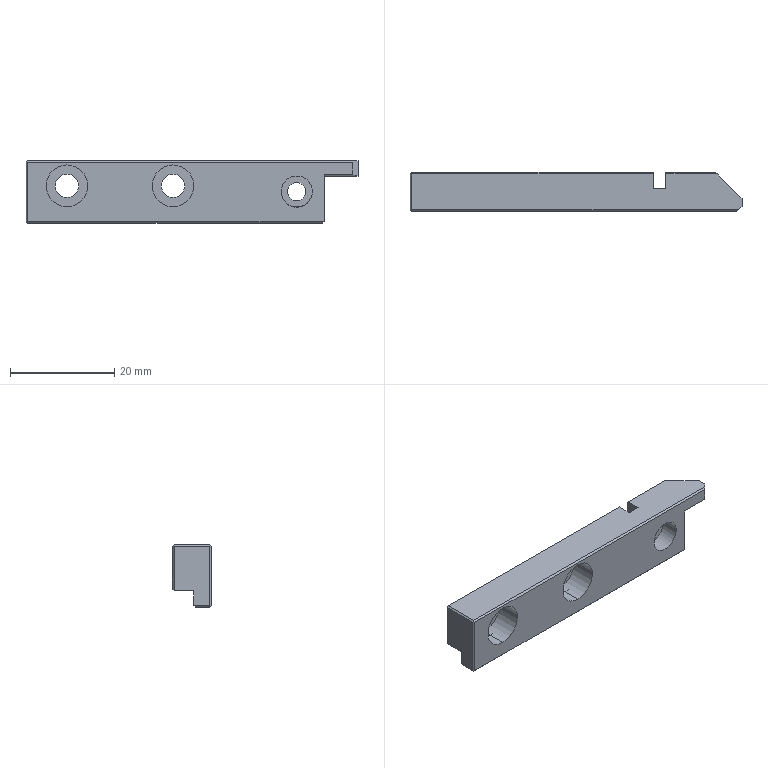Part | NX | 1 solid | 43 faces | box 63.7 x 7.5 x 11.95 mm | volume 3584 mm3 | plane 31 | cylinder 12 | commonest cylinder face diameters 4.5 x4 8 x4 3.5 x2 6 x2
STEP:
#1=CARTESIAN_POINT('',(-198.5,219.5,-37.608));
#2=VERTEX_POINT('',#1);
#3=CARTESIAN_POINT('',(-198.5,219.5,-34.742));
#4=VERTEX_POINT('',#3);
#5=CARTESIAN_POINT('',(-198.5,219.5,-36.191));
#6=DIRECTION('',(0.,0.,1.));
#7=VECTOR('',#6,1000.);
#8=LINE('',#5,#7);
#9=EDGE_CURVE('',#2,#4,#8,.T.);
#10=ORIENTED_EDGE('',*,*,#9,.T.);
#11=CARTESIAN_POINT('',(-199.2,218.8,-34.742));
#12=VERTEX_POINT('',#11);
#13=CARTESIAN_POINT('',(-196.,222.,-34.742));
#14=DIRECTION('',(0.7071,0.7071,0.));
#15=VECTOR('',#14,1000.);
#16=LINE('',#13,#15);
#17=EDGE_CURVE('',#12,#4,#16,.T.);
#18=ORIENTED_EDGE('',*,*,#17,.F.);
#19=CARTESIAN_POINT('',(-199.5,218.5,-35.042));
#20=VERTEX_POINT('',#19);
#21=CARTESIAN_POINT('',(-199.935,218.065,-35.477));
#22=DIRECTION('',(0.5774,0.5774,0.5774));
#23=VECTOR('',#22,1000.);
#24=LINE('',#21,#23);
#25=EDGE_CURVE('',#20,#12,#24,.T.);
#26=ORIENTED_EDGE('',*,*,#25,.F.);
#27=CARTESIAN_POINT('',(-199.5,218.5,-37.34));
#28=VERTEX_POINT('',#27);
#29=CARTESIAN_POINT('',(-199.5,218.5,-36.191));
#30=DIRECTION('',(0.,0.,1.));
#31=VECTOR('',#30,1000.);
#32=LINE('',#29,#31);
#33=EDGE_CURVE('',#28,#20,#32,.T.);
#34=ORIENTED_EDGE('',*,*,#33,.F.);
#35=CARTESIAN_POINT('',(-196.,222.,-38.278));
#36=DIRECTION('',(-0.6947,-0.6947,0.1862));
#37=VECTOR('',#36,1000.);
#38=LINE('',#35,#37);
#39=EDGE_CURVE('',#2,#28,#38,.T.);
#40=ORIENTED_EDGE('',*,*,#39,.F.);
#41=EDGE_LOOP('',(#10,#18,#26,#34,#40));
#42=FACE_BOUND('',#41,.T.);
#43=CARTESIAN_POINT('',(-199.,219.,-36.191));
#44=DIRECTION('',(-0.7071,0.7071,0.));
#45=DIRECTION('',(0.,0.,1.));
#46=AXIS2_PLACEMENT_3D('',#43,#44,#45);
#47=PLANE('',#46);
#48=ADVANCED_FACE('',(#42),#47,.F.);
#49=CARTESIAN_POINT('',(-262.2,218.8,-46.392));
#50=VERTEX_POINT('',#49);
#51=CARTESIAN_POINT('',(-262.2,218.8,-35.042));
#52=VERTEX_POINT('',#51);
#53=CARTESIAN_POINT('',(-262.2,218.8,-35.477));
#54=DIRECTION('',(0.,0.,1.));
#55=VECTOR('',#54,1000.);
#56=LINE('',#53,#55);
#57=EDGE_CURVE('',#50,#52,#56,.T.);
#58=ORIENTED_EDGE('',*,*,#57,.T.);
#59=CARTESIAN_POINT('',(-262.2,225.7,-35.042));
#60=VERTEX_POINT('',#59);
#61=CARTESIAN_POINT('',(-262.2,222.1,-35.042));
#62=DIRECTION('',(0.,-1.,0.));
#63=VECTOR('',#62,1000.);
#64=LINE('',#61,#63);
#65=EDGE_CURVE('',#60,#52,#64,.T.);
#66=ORIENTED_EDGE('',*,*,#65,.F.);
#67=CARTESIAN_POINT('',(-262.2,225.7,-43.542));
#68=VERTEX_POINT('',#67);
#69=CARTESIAN_POINT('',(-262.2,225.7,-39.292));
#70=DIRECTION('',(0.,0.,1.));
#71=VECTOR('',#70,1000.);
#72=LINE('',#69,#71);
#73=EDGE_CURVE('',#68,#60,#72,.T.);
#74=ORIENTED_EDGE('',*,*,#73,.F.);
#75=CARTESIAN_POINT('',(-262.2,221.9,-43.542));
#76=VERTEX_POINT('',#75);
#77=CARTESIAN_POINT('',(-262.2,222.,-43.542));
#78=DIRECTION('',(0.,1.,0.));
#79=VECTOR('',#78,1000.);
#80=LINE('',#77,#79);
#81=EDGE_CURVE('',#76,#68,#80,.T.);
#82=ORIENTED_EDGE('',*,*,#81,.F.);
#83=CARTESIAN_POINT('',(-262.2,221.9,-46.392));
#84=VERTEX_POINT('',#83);
#85=CARTESIAN_POINT('',(-262.2,221.9,-35.477));
#86=DIRECTION('',(0.,0.,1.));
#87=VECTOR('',#86,1000.);
#88=LINE('',#85,#87);
#89=EDGE_CURVE('',#84,#76,#88,.T.);
#90=ORIENTED_EDGE('',*,*,#89,.F.);
#91=CARTESIAN_POINT('',(-262.2,220.35,-46.392));
#92=DIRECTION('',(0.,-1.,0.));
#93=VECTOR('',#92,1000.);
#94=LINE('',#91,#93);
#95=EDGE_CURVE('',#84,#50,#94,.T.);
#96=ORIENTED_EDGE('',*,*,#95,.T.);
#97=EDGE_LOOP('',(#58,#66,#74,#82,#90,#96));
#98=FACE_BOUND('',#97,.T.);
#99=CARTESIAN_POINT('',(-262.2,222.,-46.8));
#100=DIRECTION('',(-1.,0.,0.));
#101=DIRECTION('',(0.,1.,0.));
#102=AXIS2_PLACEMENT_3D('',#99,#100,#101);
#103=PLANE('',#102);
#104=ADVANCED_FACE('',(#98),#103,.T.);
#105=ORIENTED_EDGE('',*,*,#9,.F.);
#106=CARTESIAN_POINT('',(-198.5,220.,-37.742));
#107=VERTEX_POINT('',#106);
#108=CARTESIAN_POINT('',(-198.5,222.,-38.278));
#109=DIRECTION('',(0.,-0.9659,0.2588));
#110=VECTOR('',#109,1000.);
#111=LINE('',#108,#110);
#112=EDGE_CURVE('',#107,#2,#111,.T.);
#113=ORIENTED_EDGE('',*,*,#112,.F.);
#114=CARTESIAN_POINT('',(-198.5,221.,-37.742));
#115=VERTEX_POINT('',#114);
#116=CARTESIAN_POINT('',(-198.5,222.,-37.742));
#117=DIRECTION('',(0.,-1.,0.));
#118=VECTOR('',#117,1000.);
#119=LINE('',#116,#118);
#120=EDGE_CURVE('',#115,#107,#119,.T.);
#121=ORIENTED_EDGE('',*,*,#120,.F.);
#122=CARTESIAN_POINT('',(-198.5,221.,-34.742));
#123=VERTEX_POINT('',#122);
#124=CARTESIAN_POINT('',(-198.5,221.,-36.392));
#125=DIRECTION('',(0.,0.,1.));
#126=VECTOR('',#125,1000.);
#127=LINE('',#124,#126);
#128=EDGE_CURVE('',#115,#123,#127,.T.);
#129=ORIENTED_EDGE('',*,*,#128,.T.);
#130=CARTESIAN_POINT('',(-198.5,222.,-34.742));
#131=DIRECTION('',(0.,1.,0.));
#132=VECTOR('',#131,1000.);
#133=LINE('',#130,#132);
#134=EDGE_CURVE('',#4,#123,#133,.T.);
#135=ORIENTED_EDGE('',*,*,#134,.F.);
#136=EDGE_LOOP('',(#105,#113,#121,#129,#135));
#137=FACE_BOUND('',#136,.T.);
#138=CARTESIAN_POINT('',(-198.5,222.,-34.));
#139=DIRECTION('',(1.,0.,0.));
#140=DIRECTION('',(0.,1.,0.));
#141=AXIS2_PLACEMENT_3D('',#138,#139,#140);
#142=PLANE('',#141);
#143=ADVANCED_FACE('',(#137),#142,.T.);
#144=CARTESIAN_POINT('',(-205.,223.,-37.742));
#145=VERTEX_POINT('',#144);
#146=CARTESIAN_POINT('',(-205.,220.,-37.742));
#147=VERTEX_POINT('',#146);
#148=CARTESIAN_POINT('',(-205.,222.,-37.742));
#149=DIRECTION('',(0.,-1.,0.));
#150=VECTOR('',#149,1000.);
#151=LINE('',#148,#150);
#152=EDGE_CURVE('',#145,#147,#151,.T.);
#153=ORIENTED_EDGE('',*,*,#152,.T.);
#154=CARTESIAN_POINT('',(-205.,218.5,-37.34));
#155=VERTEX_POINT('',#154);
#156=CARTESIAN_POINT('',(-205.,222.,-38.278));
#157=DIRECTION('',(0.,-0.9659,0.2588));
#158=VECTOR('',#157,1000.);
#159=LINE('',#156,#158);
#160=EDGE_CURVE('',#147,#155,#159,.T.);
#161=ORIENTED_EDGE('',*,*,#160,.T.);
#162=CARTESIAN_POINT('',(-205.,218.5,-46.392));
#163=VERTEX_POINT('',#162);
#164=CARTESIAN_POINT('',(-205.,218.5,-35.477));
#165=DIRECTION('',(0.,0.,-1.));
#166=VECTOR('',#165,1000.);
#167=LINE('',#164,#166);
#168=EDGE_CURVE('',#155,#163,#167,.T.);
#169=ORIENTED_EDGE('',*,*,#168,.T.);
#170=CARTESIAN_POINT('',(-205.,221.9,-46.392));
#171=VERTEX_POINT('',#170);
#172=CARTESIAN_POINT('',(-205.,220.2,-46.392));
#173=DIRECTION('',(0.,1.,0.));
#174=VECTOR('',#173,1000.);
#175=LINE('',#172,#174);
#176=EDGE_CURVE('',#163,#171,#175,.T.);
#177=ORIENTED_EDGE('',*,*,#176,.T.);
#178=CARTESIAN_POINT('',(-205.,221.9,-43.542));
#179=VERTEX_POINT('',#178);
#180=CARTESIAN_POINT('',(-205.,221.9,-35.477));
#181=DIRECTION('',(0.,0.,-1.));
#182=VECTOR('',#181,1000.);
#183=LINE('',#180,#182);
#184=EDGE_CURVE('',#179,#171,#183,.T.);
#185=ORIENTED_EDGE('',*,*,#184,.F.);
#186=CARTESIAN_POINT('',(-205.,223.,-43.542));
#187=VERTEX_POINT('',#186);
#188=CARTESIAN_POINT('',(-205.,222.,-43.542));
#189=DIRECTION('',(0.,-1.,0.));
#190=VECTOR('',#189,1000.);
#191=LINE('',#188,#190);
#192=EDGE_CURVE('',#187,#179,#191,.T.);
#193=ORIENTED_EDGE('',*,*,#192,.F.);
#194=CARTESIAN_POINT('',(-205.,223.,-35.477));
#195=DIRECTION('',(0.,0.,1.));
#196=VECTOR('',#195,1000.);
#197=LINE('',#194,#196);
#198=EDGE_CURVE('',#187,#145,#197,.T.);
#199=ORIENTED_EDGE('',*,*,#198,.T.);
#200=EDGE_LOOP('',(#153,#161,#169,#177,#185,#193,#199));
#201=FACE_BOUND('',#200,.T.);
#202=CARTESIAN_POINT('',(-205.,221.,-37.742));
#203=DIRECTION('',(1.,0.,0.));
#204=DIRECTION('',(0.,0.,1.));
#205=AXIS2_PLACEMENT_3D('',#202,#203,#204);
#206=PLANE('',#205);
#207=ADVANCED_FACE('',(#201),#206,.T.);
#208=ORIENTED_EDGE('',*,*,#134,.T.);
#209=CARTESIAN_POINT('',(-203.2,225.7,-34.742));
#210=VERTEX_POINT('',#209);
#211=CARTESIAN_POINT('',(-199.5,222.,-34.742));
#212=DIRECTION('',(-0.7071,0.7071,0.));
#213=VECTOR('',#212,1000.);
#214=LINE('',#211,#213);
#215=EDGE_CURVE('',#123,#210,#214,.T.);
#216=ORIENTED_EDGE('',*,*,#215,.T.);
#217=CARTESIAN_POINT('',(-213.1,225.7,-34.742));
#218=VERTEX_POINT('',#217);
#219=CARTESIAN_POINT('',(-222.557,225.7,-34.742));
#220=DIRECTION('',(-1.,0.,0.));
#221=VECTOR('',#220,1000.);
#222=LINE('',#219,#221);
#223=EDGE_CURVE('',#210,#218,#222,.T.);
#224=ORIENTED_EDGE('',*,*,#223,.T.);
#225=CARTESIAN_POINT('',(-213.1,223.,-34.742));
#226=VERTEX_POINT('',#225);
#227=CARTESIAN_POINT('',(-213.1,222.,-34.742));
#228=DIRECTION('',(0.,1.,0.));
#229=VECTOR('',#228,1000.);
#230=LINE('',#227,#229);
#231=EDGE_CURVE('',#226,#218,#230,.T.);
#232=ORIENTED_EDGE('',*,*,#231,.F.);
#233=CARTESIAN_POINT('',(-215.5,223.,-34.742));
#234=VERTEX_POINT('',#233);
#235=CARTESIAN_POINT('',(-222.557,223.,-34.742));
#236=DIRECTION('',(1.,0.,0.));
#237=VECTOR('',#236,1000.);
#238=LINE('',#235,#237);
#239=EDGE_CURVE('',#234,#226,#238,.T.);
#240=ORIENTED_EDGE('',*,*,#239,.F.);
#241=CARTESIAN_POINT('',(-215.5,225.7,-34.742));
#242=VERTEX_POINT('',#241);
#243=CARTESIAN_POINT('',(-215.5,222.,-34.742));
#244=DIRECTION('',(0.,-1.,0.));
#245=VECTOR('',#244,1000.);
#246=LINE('',#243,#245);
#247=EDGE_CURVE('',#242,#234,#246,.T.);
#248=ORIENTED_EDGE('',*,*,#247,.F.);
#249=CARTESIAN_POINT('',(-261.9,225.7,-34.742));
#250=VERTEX_POINT('',#249);
#251=CARTESIAN_POINT('',(-222.557,225.7,-34.742));
#252=DIRECTION('',(-1.,0.,0.));
#253=VECTOR('',#252,1000.);
#254=LINE('',#251,#253);
#255=EDGE_CURVE('',#242,#250,#254,.T.);
#256=ORIENTED_EDGE('',*,*,#255,.T.);
#257=CARTESIAN_POINT('',(-261.9,218.8,-34.742));
#258=VERTEX_POINT('',#257);
#259=CARTESIAN_POINT('',(-261.9,222.1,-34.742));
#260=DIRECTION('',(0.,-1.,0.));
#261=VECTOR('',#260,1000.);
#262=LINE('',#259,#261);
#263=EDGE_CURVE('',#250,#258,#262,.T.);
#264=ORIENTED_EDGE('',*,*,#263,.T.);
#265=CARTESIAN_POINT('',(-222.557,218.8,-34.742));
#266=DIRECTION('',(-1.,0.,0.));
#267=VECTOR('',#266,1000.);
#268=LINE('',#265,#267);
#269=EDGE_CURVE('',#12,#258,#268,.T.);
#270=ORIENTED_EDGE('',*,*,#269,.F.);
#271=ORIENTED_EDGE('',*,*,#17,.T.);
#272=EDGE_LOOP('',(#208,#216,#224,#232,#240,#248,#256,#264,#270,#271));
#273=FACE_BOUND('',#272,.T.);
#274=CARTESIAN_POINT('',(-238.1,222.,-34.742));
#275=DIRECTION('',(0.,0.,1.));
#276=DIRECTION('',(0.,-1.,0.));
#277=AXIS2_PLACEMENT_3D('',#274,#275,#276);
#278=PLANE('',#277);
#279=ADVANCED_FACE('',(#273),#278,.T.);
#280=ORIENTED_EDGE('',*,*,#57,.F.);
#281=CARTESIAN_POINT('',(-262.05,218.65,-46.542));
#282=VERTEX_POINT('',#281);
#283=CARTESIAN_POINT('',(-273.115,229.715,-35.477));
#284=DIRECTION('',(0.5774,-0.5774,-0.5774));
#285=VECTOR('',#284,1000.);
#286=LINE('',#283,#285);
#287=EDGE_CURVE('',#50,#282,#286,.T.);
#288=ORIENTED_EDGE('',*,*,#287,.T.);
#289=CARTESIAN_POINT('',(-261.9,218.5,-46.392));
#290=VERTEX_POINT('',#289);
#291=CARTESIAN_POINT('',(-250.985,207.585,-35.477));
#292=DIRECTION('',(0.5774,-0.5774,0.5774));
#293=VECTOR('',#292,1000.);
#294=LINE('',#291,#293);
#295=EDGE_CURVE('',#282,#290,#294,.T.);
#296=ORIENTED_EDGE('',*,*,#295,.T.);
#297=CARTESIAN_POINT('',(-261.9,218.5,-35.042));
#298=VERTEX_POINT('',#297);
#299=CARTESIAN_POINT('',(-261.9,218.5,-35.477));
#300=DIRECTION('',(0.,0.,1.));
#301=VECTOR('',#300,1000.);
#302=LINE('',#299,#301);
#303=EDGE_CURVE('',#290,#298,#302,.T.);
#304=ORIENTED_EDGE('',*,*,#303,.T.);
#305=CARTESIAN_POINT('',(-262.05,218.65,-34.892));
#306=VERTEX_POINT('',#305);
#307=CARTESIAN_POINT('',(-261.465,218.065,-35.477));
#308=DIRECTION('',(-0.5774,0.5774,0.5774));
#309=VECTOR('',#308,1000.);
#310=LINE('',#307,#309);
#311=EDGE_CURVE('',#298,#306,#310,.T.);
#312=ORIENTED_EDGE('',*,*,#311,.T.);
#313=CARTESIAN_POINT('',(-262.635,219.235,-35.477));
#314=DIRECTION('',(-0.5774,0.5774,-0.5774));
#315=VECTOR('',#314,1000.);
#316=LINE('',#313,#315);
#317=EDGE_CURVE('',#306,#52,#316,.T.);
#318=ORIENTED_EDGE('',*,*,#317,.T.);
#319=EDGE_LOOP('',(#280,#288,#296,#304,#312,#318));
#320=FACE_BOUND('',#319,.T.);
#321=CARTESIAN_POINT('',(-262.05,218.65,-40.992));
#322=DIRECTION('',(-0.7071,-0.7071,0.));
#323=DIRECTION('',(-0.7071,0.7071,0.));
#324=AXIS2_PLACEMENT_3D('',#321,#322,#323);
#325=PLANE('',#324);
#326=ADVANCED_FACE('',(#320),#325,.T.);
#327=CARTESIAN_POINT('',(-215.5,223.,-43.542));
#328=VERTEX_POINT('',#327);
#329=CARTESIAN_POINT('',(-222.557,223.,-43.542));
#330=DIRECTION('',(1.,0.,0.));
#331=VECTOR('',#330,1000.);
#332=LINE('',#329,#331);
#333=EDGE_CURVE('',#328,#187,#332,.T.);
#334=ORIENTED_EDGE('',*,*,#333,.T.);
#335=ORIENTED_EDGE('',*,*,#192,.T.);
#336=CARTESIAN_POINT('',(-209.482,221.9,-43.542));
#337=VERTEX_POINT('',#336);
#338=CARTESIAN_POINT('',(-222.557,221.9,-43.542));
#339=DIRECTION('',(-1.,0.,0.));
#340=VECTOR('',#339,1000.);
#341=LINE('',#338,#340);
#342=EDGE_CURVE('',#179,#337,#341,.T.);
#343=ORIENTED_EDGE('',*,*,#342,.T.);
#344=CARTESIAN_POINT('',(-209.482,222.,-43.542));
#345=VERTEX_POINT('',#344);
#346=CARTESIAN_POINT('',(-209.482,218.5,-43.542));
#347=DIRECTION('',(0.,-1.,0.));
#348=VECTOR('',#347,1000.);
#349=LINE('',#346,#348);
#350=EDGE_CURVE('',#345,#337,#349,.T.);
#351=ORIENTED_EDGE('',*,*,#350,.F.);
#352=CARTESIAN_POINT('',(-211.018,222.,-43.542));
#353=VERTEX_POINT('',#352);
#354=CARTESIAN_POINT('',(-222.557,222.,-43.542));
#355=DIRECTION('',(1.,0.,0.));
#356=VECTOR('',#355,1000.);
#357=LINE('',#354,#356);
#358=EDGE_CURVE('',#353,#345,#357,.T.);
#359=ORIENTED_EDGE('',*,*,#358,.F.);
#360=CARTESIAN_POINT('',(-211.018,221.9,-43.542));
#361=VERTEX_POINT('',#360);
#362=CARTESIAN_POINT('',(-211.018,218.5,-43.542));
#363=DIRECTION('',(0.,-1.,0.));
#364=VECTOR('',#363,1000.);
#365=LINE('',#362,#364);
#366=EDGE_CURVE('',#353,#361,#365,.T.);
#367=ORIENTED_EDGE('',*,*,#366,.T.);
#368=CARTESIAN_POINT('',(-222.557,221.9,-43.542));
#369=DIRECTION('',(-1.,0.,0.));
#370=VECTOR('',#369,1000.);
#371=LINE('',#368,#370);
#372=EDGE_CURVE('',#361,#76,#371,.T.);
#373=ORIENTED_EDGE('',*,*,#372,.T.);
#374=ORIENTED_EDGE('',*,*,#81,.T.);
#375=CARTESIAN_POINT('',(-215.5,225.7,-43.542));
#376=VERTEX_POINT('',#375);
#377=CARTESIAN_POINT('',(-233.45,225.7,-43.542));
#378=DIRECTION('',(1.,0.,0.));
#379=VECTOR('',#378,1000.);
#380=LINE('',#377,#379);
#381=EDGE_CURVE('',#68,#376,#380,.T.);
#382=ORIENTED_EDGE('',*,*,#381,.T.);
#383=CARTESIAN_POINT('',(-215.5,222.,-43.542));
#384=DIRECTION('',(0.,-1.,0.));
#385=VECTOR('',#384,1000.);
#386=LINE('',#383,#385);
#387=EDGE_CURVE('',#376,#328,#386,.T.);
#388=ORIENTED_EDGE('',*,*,#387,.T.);
#389=EDGE_LOOP('',(#334,#335,#343,#351,#359,#367,#373,#374,#382,#388));
#390=FACE_BOUND('',#389,.T.);
#391=CARTESIAN_POINT('',(-193.78,226.,-43.542));
#392=DIRECTION('',(0.,0.,1.));
#393=DIRECTION('',(1.,0.,0.));
#394=AXIS2_PLACEMENT_3D('',#391,#392,#393);
#395=PLANE('',#394);
#396=ADVANCED_FACE('',(#390),#395,.F.);
#397=CARTESIAN_POINT('',(-215.5,226.,-43.242));
#398=VERTEX_POINT('',#397);
#399=CARTESIAN_POINT('',(-215.5,222.,-47.242));
#400=DIRECTION('',(0.,0.7071,0.7071));
#401=VECTOR('',#400,1000.);
#402=LINE('',#399,#401);
#403=EDGE_CURVE('',#376,#398,#402,.T.);
#404=ORIENTED_EDGE('',*,*,#403,.F.);
#405=ORIENTED_EDGE('',*,*,#381,.F.);
#406=CARTESIAN_POINT('',(-261.9,226.,-43.242));
#407=VERTEX_POINT('',#406);
#408=CARTESIAN_POINT('',(-265.9,222.,-47.242));
#409=DIRECTION('',(0.5774,0.5774,0.5774));
#410=VECTOR('',#409,1000.);
#411=LINE('',#408,#410);
#412=EDGE_CURVE('',#68,#407,#411,.T.);
#413=ORIENTED_EDGE('',*,*,#412,.T.);
#414=CARTESIAN_POINT('',(-233.45,226.,-43.242));
#415=DIRECTION('',(1.,0.,0.));
#416=VECTOR('',#415,1000.);
#417=LINE('',#414,#416);
#418=EDGE_CURVE('',#407,#398,#417,.T.);
#419=ORIENTED_EDGE('',*,*,#418,.T.);
#420=EDGE_LOOP('',(#404,#405,#413,#419));
#421=FACE_BOUND('',#420,.T.);
#422=CARTESIAN_POINT('',(-233.45,225.85,-43.392));
#423=DIRECTION('',(0.,0.7071,-0.7071));
#424=DIRECTION('',(-1.,0.,0.));
#425=AXIS2_PLACEMENT_3D('',#422,#423,#424);
#426=PLANE('',#425);
#427=ADVANCED_FACE('',(#421),#426,.T.);
#428=ORIENTED_EDGE('',*,*,#89,.T.);
#429=ORIENTED_EDGE('',*,*,#372,.F.);
#430=CARTESIAN_POINT('',(-210.25,221.9,-40.642));
#431=DIRECTION('',(0.,-1.,0.));
#432=DIRECTION('',(1.,0.,0.));
#433=AXIS2_PLACEMENT_3D('',#430,#431,#432);
#434=CIRCLE('',#433,3.);
#435=EDGE_CURVE('',#361,#337,#434,.T.);
#436=ORIENTED_EDGE('',*,*,#435,.T.);
#437=ORIENTED_EDGE('',*,*,#342,.F.);
#438=ORIENTED_EDGE('',*,*,#184,.T.);
#439=CARTESIAN_POINT('',(-233.6,221.9,-46.392));
#440=DIRECTION('',(1.,0.,0.));
#441=VECTOR('',#440,1000.);
#442=LINE('',#439,#441);
#443=EDGE_CURVE('',#84,#171,#442,.T.);
#444=ORIENTED_EDGE('',*,*,#443,.F.);
#445=EDGE_LOOP('',(#428,#429,#436,#437,#438,#444));
#446=FACE_BOUND('',#445,.T.);
#447=CARTESIAN_POINT('',(-193.78,221.9,-44.342));
#448=DIRECTION('',(0.,-1.,0.));
#449=DIRECTION('',(0.,0.,-1.));
#450=AXIS2_PLACEMENT_3D('',#447,#448,#449);
#451=PLANE('',#450);
#452=ADVANCED_FACE('',(#446),#451,.F.);
#453=ORIENTED_EDGE('',*,*,#263,.F.);
#454=CARTESIAN_POINT('',(-262.05,225.85,-34.892));
#455=VERTEX_POINT('',#454);
#456=CARTESIAN_POINT('',(-262.635,226.435,-35.477));
#457=DIRECTION('',(-0.5774,0.5774,-0.5774));
#458=VECTOR('',#457,1000.);
#459=LINE('',#456,#458);
#460=EDGE_CURVE('',#250,#455,#459,.T.);
#461=ORIENTED_EDGE('',*,*,#460,.T.);
#462=CARTESIAN_POINT('',(-262.635,225.265,-35.477));
#463=DIRECTION('',(0.5774,0.5774,0.5774));
#464=VECTOR('',#463,1000.);
#465=LINE('',#462,#464);
#466=EDGE_CURVE('',#60,#455,#465,.T.);
#467=ORIENTED_EDGE('',*,*,#466,.F.);
#468=ORIENTED_EDGE('',*,*,#65,.T.);
#469=ORIENTED_EDGE('',*,*,#317,.F.);
#470=CARTESIAN_POINT('',(-262.635,218.065,-35.477));
#471=DIRECTION('',(0.5774,0.5774,0.5774));
#472=VECTOR('',#471,1000.);
#473=LINE('',#470,#472);
#474=EDGE_CURVE('',#306,#258,#473,.T.);
#475=ORIENTED_EDGE('',*,*,#474,.T.);
#476=EDGE_LOOP('',(#453,#461,#467,#468,#469,#475));
#477=FACE_BOUND('',#476,.T.);
#478=CARTESIAN_POINT('',(-262.05,222.1,-34.892));
#479=DIRECTION('',(-0.7071,0.,0.7071));
#480=DIRECTION('',(0.,1.,0.));
#481=AXIS2_PLACEMENT_3D('',#478,#479,#480);
#482=PLANE('',#481);
#483=ADVANCED_FACE('',(#477),#482,.T.);
#484=CARTESIAN_POINT('',(-213.25,218.5,-40.642));
#485=VERTEX_POINT('',#484);
#486=CARTESIAN_POINT('',(-207.25,218.5,-40.642));
#487=VERTEX_POINT('',#486);
#488=CARTESIAN_POINT('',(-210.25,218.5,-40.642));
#489=DIRECTION('',(0.,-1.,0.));
#490=DIRECTION('',(1.,0.,0.));
#491=AXIS2_PLACEMENT_3D('',#488,#489,#490);
#492=CIRCLE('',#491,3.);
#493=EDGE_CURVE('',#485,#487,#492,.T.);
#494=ORIENTED_EDGE('',*,*,#493,.T.);
#495=CARTESIAN_POINT('',(-207.25,222.,-40.642));
#496=VERTEX_POINT('',#495);
#497=CARTESIAN_POINT('',(-207.25,218.5,-40.642));
#498=DIRECTION('',(0.,-1.,0.));
#499=VECTOR('',#498,1000.);
#500=LINE('',#497,#499);
#501=EDGE_CURVE('',#496,#487,#500,.T.);
#502=ORIENTED_EDGE('',*,*,#501,.F.);
#503=CARTESIAN_POINT('',(-210.25,222.,-40.642));
#504=DIRECTION('',(0.,-1.,0.));
#505=DIRECTION('',(1.,0.,0.));
#506=AXIS2_PLACEMENT_3D('',#503,#504,#505);
#507=CIRCLE('',#506,3.);
#508=EDGE_CURVE('',#345,#496,#507,.T.);
#509=ORIENTED_EDGE('',*,*,#508,.F.);
#510=ORIENTED_EDGE('',*,*,#350,.T.);
#511=ORIENTED_EDGE('',*,*,#435,.F.);
#512=ORIENTED_EDGE('',*,*,#366,.F.);
#513=CARTESIAN_POINT('',(-213.25,222.,-40.642));
#514=VERTEX_POINT('',#513);
#515=CARTESIAN_POINT('',(-210.25,222.,-40.642));
#516=DIRECTION('',(0.,-1.,0.));
#517=DIRECTION('',(1.,0.,0.));
#518=AXIS2_PLACEMENT_3D('',#515,#516,#517);
#519=CIRCLE('',#518,3.);
#520=EDGE_CURVE('',#514,#353,#519,.T.);
#521=ORIENTED_EDGE('',*,*,#520,.F.);
#522=CARTESIAN_POINT('',(-213.25,218.5,-40.642));
#523=DIRECTION('',(0.,-1.,0.));
#524=VECTOR('',#523,1000.);
#525=LINE('',#522,#524);
#526=EDGE_CURVE('',#514,#485,#525,.T.);
#527=ORIENTED_EDGE('',*,*,#526,.T.);
#528=EDGE_LOOP('',(#494,#502,#509,#510,#511,#512,#521,#527));
#529=FACE_BOUND('',#528,.T.);
#530=CARTESIAN_POINT('',(-210.25,218.5,-40.642));
#531=DIRECTION('',(0.,-1.,0.));
#532=DIRECTION('',(1.,0.,0.));
#533=AXIS2_PLACEMENT_3D('',#530,#531,#532);
#534=CYLINDRICAL_SURFACE('',#533,3.);
#535=ADVANCED_FACE('',(#529),#534,.F.);
#536=ORIENTED_EDGE('',*,*,#520,.T.);
#537=ORIENTED_EDGE('',*,*,#358,.T.);
#538=ORIENTED_EDGE('',*,*,#508,.T.);
#539=CARTESIAN_POINT('',(-210.25,222.,-40.642));
#540=DIRECTION('',(0.,-1.,0.));
#541=DIRECTION('',(1.,0.,0.));
#542=AXIS2_PLACEMENT_3D('',#539,#540,#541);
#543=CIRCLE('',#542,3.);
#544=EDGE_CURVE('',#496,#514,#543,.T.);
#545=ORIENTED_EDGE('',*,*,#544,.T.);
#546=EDGE_LOOP('',(#536,#537,#538,#545));
#547=FACE_BOUND('',#546,.T.);
#548=CARTESIAN_POINT('',(-212.,222.,-40.642));
#549=VERTEX_POINT('',#548);
#550=CARTESIAN_POINT('',(-208.5,222.,-40.642));
#551=VERTEX_POINT('',#550);
#552=CARTESIAN_POINT('',(-210.25,222.,-40.642));
#553=DIRECTION('',(0.,-1.,0.));
#554=DIRECTION('',(1.,0.,0.));
#555=AXIS2_PLACEMENT_3D('',#552,#553,#554);
#556=CIRCLE('',#555,1.75);
#557=EDGE_CURVE('',#549,#551,#556,.T.);
#558=ORIENTED_EDGE('',*,*,#557,.F.);
#559=CARTESIAN_POINT('',(-210.25,222.,-40.642));
#560=DIRECTION('',(0.,-1.,0.));
#561=DIRECTION('',(1.,0.,0.));
#562=AXIS2_PLACEMENT_3D('',#559,#560,#561);
#563=CIRCLE('',#562,1.75);
#564=EDGE_CURVE('',#551,#549,#563,.T.);
#565=ORIENTED_EDGE('',*,*,#564,.F.);
#566=EDGE_LOOP('',(#558,#565));
#567=FACE_BOUND('',#566,.T.);
#568=CARTESIAN_POINT('',(-210.25,222.,-40.642));
#569=DIRECTION('',(0.,-1.,0.));
#570=DIRECTION('',(0.,0.,-1.));
#571=AXIS2_PLACEMENT_3D('',#568,#569,#570);
#572=PLANE('',#571);
#573=ADVANCED_FACE('',(#547,#567),#572,.T.);
#574=ORIENTED_EDGE('',*,*,#557,.T.);
#575=CARTESIAN_POINT('',(-208.5,223.,-40.642));
#576=VERTEX_POINT('',#575);
#577=CARTESIAN_POINT('',(-208.5,218.5,-40.642));
#578=DIRECTION('',(0.,-1.,0.));
#579=VECTOR('',#578,1000.);
#580=LINE('',#577,#579);
#581=EDGE_CURVE('',#576,#551,#580,.T.);
#582=ORIENTED_EDGE('',*,*,#581,.F.);
#583=CARTESIAN_POINT('',(-212.,223.,-40.642));
#584=VERTEX_POINT('',#583);
#585=CARTESIAN_POINT('',(-210.25,223.,-40.642));
#586=DIRECTION('',(0.,-1.,0.));
#587=DIRECTION('',(1.,0.,0.));
#588=AXIS2_PLACEMENT_3D('',#585,#586,#587);
#589=CIRCLE('',#588,1.75);
#590=EDGE_CURVE('',#584,#576,#589,.T.);
#591=ORIENTED_EDGE('',*,*,#590,.F.);
#592=CARTESIAN_POINT('',(-212.,218.5,-40.642));
#593=DIRECTION('',(0.,-1.,0.));
#594=VECTOR('',#593,1000.);
#595=LINE('',#592,#594);
#596=EDGE_CURVE('',#584,#549,#595,.T.);
#597=ORIENTED_EDGE('',*,*,#596,.T.);
#598=EDGE_LOOP('',(#574,#582,#591,#597));
#599=FACE_BOUND('',#598,.T.);
#600=CARTESIAN_POINT('',(-210.25,218.5,-40.642));
#601=DIRECTION('',(0.,-1.,0.));
#602=DIRECTION('',(1.,0.,0.));
#603=AXIS2_PLACEMENT_3D('',#600,#601,#602);
#604=CYLINDRICAL_SURFACE('',#603,1.75);
#605=ADVANCED_FACE('',(#599),#604,.F.);
#606=ORIENTED_EDGE('',*,*,#501,.T.);
#607=CARTESIAN_POINT('',(-210.25,218.5,-40.642));
#608=DIRECTION('',(0.,-1.,0.));
#609=DIRECTION('',(1.,0.,0.));
#610=AXIS2_PLACEMENT_3D('',#607,#608,#609);
#611=CIRCLE('',#610,3.);
#612=EDGE_CURVE('',#487,#485,#611,.T.);
#613=ORIENTED_EDGE('',*,*,#612,.T.);
#614=ORIENTED_EDGE('',*,*,#526,.F.);
#615=ORIENTED_EDGE('',*,*,#544,.F.);
#616=EDGE_LOOP('',(#606,#613,#614,#615));
#617=FACE_BOUND('',#616,.T.);
#618=CARTESIAN_POINT('',(-210.25,218.5,-40.642));
#619=DIRECTION('',(0.,-1.,0.));
#620=DIRECTION('',(1.,0.,0.));
#621=AXIS2_PLACEMENT_3D('',#618,#619,#620);
#622=CYLINDRICAL_SURFACE('',#621,3.);
#623=ADVANCED_FACE('',(#617),#622,.F.);
#624=ORIENTED_EDGE('',*,*,#581,.T.);
#625=ORIENTED_EDGE('',*,*,#564,.T.);
#626=ORIENTED_EDGE('',*,*,#596,.F.);
#627=CARTESIAN_POINT('',(-210.25,223.,-40.642));
#628=DIRECTION('',(0.,-1.,0.));
#629=DIRECTION('',(1.,0.,0.));
#630=AXIS2_PLACEMENT_3D('',#627,#628,#629);
#631=CIRCLE('',#630,1.75);
#632=EDGE_CURVE('',#576,#584,#631,.T.);
#633=ORIENTED_EDGE('',*,*,#632,.F.);
#634=EDGE_LOOP('',(#624,#625,#626,#633));
#635=FACE_BOUND('',#634,.T.);
#636=CARTESIAN_POINT('',(-210.25,218.5,-40.642));
#637=DIRECTION('',(0.,-1.,0.));
#638=DIRECTION('',(1.,0.,0.));
#639=AXIS2_PLACEMENT_3D('',#636,#637,#638);
#640=CYLINDRICAL_SURFACE('',#639,1.75);
#641=ADVANCED_FACE('',(#635),#640,.F.);
#642=CARTESIAN_POINT('',(-222.557,218.5,-35.042));
#643=DIRECTION('',(-1.,0.,0.));
#644=VECTOR('',#643,1000.);
#645=LINE('',#642,#644);
#646=EDGE_CURVE('',#20,#298,#645,.T.);
#647=ORIENTED_EDGE('',*,*,#646,.T.);
#648=ORIENTED_EDGE('',*,*,#303,.F.);
#649=CARTESIAN_POINT('',(-233.45,218.5,-46.392));
#650=DIRECTION('',(1.,0.,0.));
#651=VECTOR('',#650,1000.);
#652=LINE('',#649,#651);
#653=EDGE_CURVE('',#290,#163,#652,.T.);
#654=ORIENTED_EDGE('',*,*,#653,.T.);
#655=ORIENTED_EDGE('',*,*,#168,.F.);
#656=CARTESIAN_POINT('',(-222.557,218.5,-37.34));
#657=DIRECTION('',(1.,0.,0.));
#658=VECTOR('',#657,1000.);
#659=LINE('',#656,#658);
#660=EDGE_CURVE('',#155,#28,#659,.T.);
#661=ORIENTED_EDGE('',*,*,#660,.T.);
#662=ORIENTED_EDGE('',*,*,#33,.T.);
#663=EDGE_LOOP('',(#647,#648,#654,#655,#661,#662));
#664=FACE_BOUND('',#663,.T.);
#665=CARTESIAN_POINT('',(-234.,218.5,-43.529));
#666=VERTEX_POINT('',#665);
#667=CARTESIAN_POINT('',(-234.,218.5,-35.529));
#668=VERTEX_POINT('',#667);
#669=CARTESIAN_POINT('',(-234.,218.5,-39.529));
#670=DIRECTION('',(0.,-1.,0.));
#671=DIRECTION('',(0.,0.,1.));
#672=AXIS2_PLACEMENT_3D('',#669,#670,#671);
#673=CIRCLE('',#672,4.);
#674=EDGE_CURVE('',#666,#668,#673,.T.);
#675=ORIENTED_EDGE('',*,*,#674,.F.);
#676=CARTESIAN_POINT('',(-234.,218.5,-39.529));
#677=DIRECTION('',(0.,-1.,0.));
#678=DIRECTION('',(0.,0.,1.));
#679=AXIS2_PLACEMENT_3D('',#676,#677,#678);
#680=CIRCLE('',#679,4.);
#681=EDGE_CURVE('',#668,#666,#680,.T.);
#682=ORIENTED_EDGE('',*,*,#681,.F.);
#683=EDGE_LOOP('',(#675,#682));
#684=FACE_BOUND('',#683,.T.);
#685=CARTESIAN_POINT('',(-254.35,218.5,-43.529));
#686=VERTEX_POINT('',#685);
#687=CARTESIAN_POINT('',(-254.35,218.5,-35.529));
#688=VERTEX_POINT('',#687);
#689=CARTESIAN_POINT('',(-254.35,218.5,-39.529));
#690=DIRECTION('',(0.,-1.,0.));
#691=DIRECTION('',(0.,0.,1.));
#692=AXIS2_PLACEMENT_3D('',#689,#690,#691);
#693=CIRCLE('',#692,4.);
#694=EDGE_CURVE('',#686,#688,#693,.T.);
#695=ORIENTED_EDGE('',*,*,#694,.F.);
#696=CARTESIAN_POINT('',(-254.35,218.5,-39.529));
#697=DIRECTION('',(0.,-1.,0.));
#698=DIRECTION('',(0.,0.,1.));
#699=AXIS2_PLACEMENT_3D('',#696,#697,#698);
#700=CIRCLE('',#699,4.);
#701=EDGE_CURVE('',#688,#686,#700,.T.);
#702=ORIENTED_EDGE('',*,*,#701,.F.);
#703=EDGE_LOOP('',(#695,#702));
#704=FACE_BOUND('',#703,.T.);
#705=ORIENTED_EDGE('',*,*,#493,.F.);
#706=ORIENTED_EDGE('',*,*,#612,.F.);
#707=EDGE_LOOP('',(#705,#706));
#708=FACE_BOUND('',#707,.T.);
#709=CARTESIAN_POINT('',(-222.557,218.5,-35.477));
#710=DIRECTION('',(0.,-1.,0.));
#711=DIRECTION('',(0.,0.,-1.));
#712=AXIS2_PLACEMENT_3D('',#709,#710,#711);
#713=PLANE('',#712);
#714=ADVANCED_FACE('',(#664,#684,#704,#708),#713,.T.);
#715=CARTESIAN_POINT('',(-261.9,221.6,-46.692));
#716=VERTEX_POINT('',#715);
#717=CARTESIAN_POINT('',(-205.3,221.6,-46.692));
#718=VERTEX_POINT('',#717);
#719=CARTESIAN_POINT('',(-233.6,221.6,-46.692));
#720=DIRECTION('',(1.,0.,0.));
#721=VECTOR('',#720,1000.);
#722=LINE('',#719,#721);
#723=EDGE_CURVE('',#716,#718,#722,.T.);
#724=ORIENTED_EDGE('',*,*,#723,.T.);
#725=CARTESIAN_POINT('',(-205.3,218.8,-46.692));
#726=VERTEX_POINT('',#725);
#727=CARTESIAN_POINT('',(-205.3,220.2,-46.692));
#728=DIRECTION('',(0.,1.,0.));
#729=VECTOR('',#728,1000.);
#730=LINE('',#727,#729);
#731=EDGE_CURVE('',#726,#718,#730,.T.);
#732=ORIENTED_EDGE('',*,*,#731,.F.);
#733=CARTESIAN_POINT('',(-261.9,218.8,-46.692));
#734=VERTEX_POINT('',#733);
#735=CARTESIAN_POINT('',(-233.45,218.8,-46.692));
#736=DIRECTION('',(1.,0.,0.));
#737=VECTOR('',#736,1000.);
#738=LINE('',#735,#737);
#739=EDGE_CURVE('',#734,#726,#738,.T.);
#740=ORIENTED_EDGE('',*,*,#739,.F.);
#741=CARTESIAN_POINT('',(-261.9,220.35,-46.692));
#742=DIRECTION('',(0.,-1.,0.));
#743=VECTOR('',#742,1000.);
#744=LINE('',#741,#743);
#745=EDGE_CURVE('',#716,#734,#744,.T.);
#746=ORIENTED_EDGE('',*,*,#745,.F.);
#747=EDGE_LOOP('',(#724,#732,#740,#746));
#748=FACE_BOUND('',#747,.T.);
#749=CARTESIAN_POINT('',(-211.32,224.131,-46.692));
#750=DIRECTION('',(0.,0.,-1.));
#751=DIRECTION('',(-1.,0.,0.));
#752=AXIS2_PLACEMENT_3D('',#749,#750,#751);
#753=PLANE('',#752);
#754=ADVANCED_FACE('',(#748),#753,.T.);
#755=CARTESIAN_POINT('',(-254.35,223.5,-41.779));
#756=VERTEX_POINT('',#755);
#757=CARTESIAN_POINT('',(-254.35,223.5,-37.279));
#758=VERTEX_POINT('',#757);
#759=CARTESIAN_POINT('',(-254.35,223.5,-39.529));
#760=DIRECTION('',(0.,-1.,0.));
#761=DIRECTION('',(0.,0.,1.));
#762=AXIS2_PLACEMENT_3D('',#759,#760,#761);
#763=CIRCLE('',#762,2.25);
#764=EDGE_CURVE('',#756,#758,#763,.T.);
#765=ORIENTED_EDGE('',*,*,#764,.T.);
#766=CARTESIAN_POINT('',(-254.35,226.,-37.279));
#767=VERTEX_POINT('',#766);
#768=CARTESIAN_POINT('',(-254.35,218.,-37.279));
#769=DIRECTION('',(0.,-1.,0.));
#770=VECTOR('',#769,1000.);
#771=LINE('',#768,#770);
#772=EDGE_CURVE('',#767,#758,#771,.T.);
#773=ORIENTED_EDGE('',*,*,#772,.F.);
#774=CARTESIAN_POINT('',(-254.35,226.,-41.779));
#775=VERTEX_POINT('',#774);
#776=CARTESIAN_POINT('',(-254.35,226.,-39.529));
#777=DIRECTION('',(0.,-1.,0.));
#778=DIRECTION('',(0.,0.,1.));
#779=AXIS2_PLACEMENT_3D('',#776,#777,#778);
#780=CIRCLE('',#779,2.25);
#781=EDGE_CURVE('',#775,#767,#780,.T.);
#782=ORIENTED_EDGE('',*,*,#781,.F.);
#783=CARTESIAN_POINT('',(-254.35,218.,-41.779));
#784=DIRECTION('',(0.,-1.,0.));
#785=VECTOR('',#784,1000.);
#786=LINE('',#783,#785);
#787=EDGE_CURVE('',#775,#756,#786,.T.);
#788=ORIENTED_EDGE('',*,*,#787,.T.);
#789=EDGE_LOOP('',(#765,#773,#782,#788));
#790=FACE_BOUND('',#789,.T.);
#791=CARTESIAN_POINT('',(-254.35,218.,-39.529));
#792=DIRECTION('',(0.,-1.,0.));
#793=DIRECTION('',(0.,0.,1.));
#794=AXIS2_PLACEMENT_3D('',#791,#792,#793);
#795=CYLINDRICAL_SURFACE('',#794,2.25);
#796=ADVANCED_FACE('',(#790),#795,.F.);
#797=CARTESIAN_POINT('',(-234.,223.5,-43.529));
#798=VERTEX_POINT('',#797);
#799=CARTESIAN_POINT('',(-234.,223.5,-35.529));
#800=VERTEX_POINT('',#799);
#801=CARTESIAN_POINT('',(-234.,223.5,-39.529));
#802=DIRECTION('',(0.,-1.,0.));
#803=DIRECTION('',(0.,0.,1.));
#804=AXIS2_PLACEMENT_3D('',#801,#802,#803);
#805=CIRCLE('',#804,4.);
#806=EDGE_CURVE('',#798,#800,#805,.T.);
#807=ORIENTED_EDGE('',*,*,#806,.T.);
#808=CARTESIAN_POINT('',(-234.,223.5,-39.529));
#809=DIRECTION('',(0.,-1.,0.));
#810=DIRECTION('',(0.,0.,1.));
#811=AXIS2_PLACEMENT_3D('',#808,#809,#810);
#812=CIRCLE('',#811,4.);
#813=EDGE_CURVE('',#800,#798,#812,.T.);
#814=ORIENTED_EDGE('',*,*,#813,.T.);
#815=EDGE_LOOP('',(#807,#814));
#816=FACE_BOUND('',#815,.T.);
#817=CARTESIAN_POINT('',(-234.,223.5,-41.779));
#818=VERTEX_POINT('',#817);
#819=CARTESIAN_POINT('',(-234.,223.5,-37.279));
#820=VERTEX_POINT('',#819);
#821=CARTESIAN_POINT('',(-234.,223.5,-39.529));
#822=DIRECTION('',(0.,-1.,0.));
#823=DIRECTION('',(0.,0.,1.));
#824=AXIS2_PLACEMENT_3D('',#821,#822,#823);
#825=CIRCLE('',#824,2.25);
#826=EDGE_CURVE('',#818,#820,#825,.T.);
#827=ORIENTED_EDGE('',*,*,#826,.F.);
#828=CARTESIAN_POINT('',(-234.,223.5,-39.529));
#829=DIRECTION('',(0.,-1.,0.));
#830=DIRECTION('',(0.,0.,1.));
#831=AXIS2_PLACEMENT_3D('',#828,#829,#830);
#832=CIRCLE('',#831,2.25);
#833=EDGE_CURVE('',#820,#818,#832,.T.);
#834=ORIENTED_EDGE('',*,*,#833,.F.);
#835=EDGE_LOOP('',(#827,#834));
#836=FACE_BOUND('',#835,.T.);
#837=CARTESIAN_POINT('',(-234.,223.5,-39.529));
#838=DIRECTION('',(0.,-1.,0.));
#839=DIRECTION('',(0.,0.,-1.));
#840=AXIS2_PLACEMENT_3D('',#837,#838,#839);
#841=PLANE('',#840);
#842=ADVANCED_FACE('',(#816,#836),#841,.T.);
#843=ORIENTED_EDGE('',*,*,#826,.T.);
#844=CARTESIAN_POINT('',(-234.,226.,-37.279));
#845=VERTEX_POINT('',#844);
#846=CARTESIAN_POINT('',(-234.,218.,-37.279));
#847=DIRECTION('',(0.,-1.,0.));
#848=VECTOR('',#847,1000.);
#849=LINE('',#846,#848);
#850=EDGE_CURVE('',#845,#820,#849,.T.);
#851=ORIENTED_EDGE('',*,*,#850,.F.);
#852=CARTESIAN_POINT('',(-234.,226.,-41.779));
#853=VERTEX_POINT('',#852);
#854=CARTESIAN_POINT('',(-234.,226.,-39.529));
#855=DIRECTION('',(0.,-1.,0.));
#856=DIRECTION('',(0.,0.,1.));
#857=AXIS2_PLACEMENT_3D('',#854,#855,#856);
#858=CIRCLE('',#857,2.25);
#859=EDGE_CURVE('',#853,#845,#858,.T.);
#860=ORIENTED_EDGE('',*,*,#859,.F.);
#861=CARTESIAN_POINT('',(-234.,218.,-41.779));
#862=DIRECTION('',(0.,-1.,0.));
#863=VECTOR('',#862,1000.);
#864=LINE('',#861,#863);
#865=EDGE_CURVE('',#853,#818,#864,.T.);
#866=ORIENTED_EDGE('',*,*,#865,.T.);
#867=EDGE_LOOP('',(#843,#851,#860,#866));
#868=FACE_BOUND('',#867,.T.);
#869=CARTESIAN_POINT('',(-234.,218.,-39.529));
#870=DIRECTION('',(0.,-1.,0.));
#871=DIRECTION('',(0.,0.,1.));
#872=AXIS2_PLACEMENT_3D('',#869,#870,#871);
#873=CYLINDRICAL_SURFACE('',#872,2.25);
#874=ADVANCED_FACE('',(#868),#873,.F.);
#875=ORIENTED_EDGE('',*,*,#674,.T.);
#876=CARTESIAN_POINT('',(-234.,218.,-35.529));
#877=DIRECTION('',(0.,-1.,0.));
#878=VECTOR('',#877,1000.);
#879=LINE('',#876,#878);
#880=EDGE_CURVE('',#800,#668,#879,.T.);
#881=ORIENTED_EDGE('',*,*,#880,.F.);
#882=ORIENTED_EDGE('',*,*,#806,.F.);
#883=CARTESIAN_POINT('',(-234.,218.,-43.529));
#884=DIRECTION('',(0.,-1.,0.));
#885=VECTOR('',#884,1000.);
#886=LINE('',#883,#885);
#887=EDGE_CURVE('',#798,#666,#886,.T.);
#888=ORIENTED_EDGE('',*,*,#887,.T.);
#889=EDGE_LOOP('',(#875,#881,#882,#888));
#890=FACE_BOUND('',#889,.T.);
#891=CARTESIAN_POINT('',(-234.,218.,-39.529));
#892=DIRECTION('',(0.,-1.,0.));
#893=DIRECTION('',(0.,0.,1.));
#894=AXIS2_PLACEMENT_3D('',#891,#892,#893);
#895=CYLINDRICAL_SURFACE('',#894,4.);
#896=ADVANCED_FACE('',(#890),#895,.F.);
#897=ORIENTED_EDGE('',*,*,#694,.T.);
#898=CARTESIAN_POINT('',(-254.35,223.5,-35.529));
#899=VERTEX_POINT('',#898);
#900=CARTESIAN_POINT('',(-254.35,218.,-35.529));
#901=DIRECTION('',(0.,-1.,0.));
#902=VECTOR('',#901,1000.);
#903=LINE('',#900,#902);
#904=EDGE_CURVE('',#899,#688,#903,.T.);
#905=ORIENTED_EDGE('',*,*,#904,.F.);
#906=CARTESIAN_POINT('',(-254.35,223.5,-43.529));
#907=VERTEX_POINT('',#906);
#908=CARTESIAN_POINT('',(-254.35,223.5,-39.529));
#909=DIRECTION('',(0.,-1.,0.));
#910=DIRECTION('',(0.,0.,1.));
#911=AXIS2_PLACEMENT_3D('',#908,#909,#910);
#912=CIRCLE('',#911,4.);
#913=EDGE_CURVE('',#907,#899,#912,.T.);
#914=ORIENTED_EDGE('',*,*,#913,.F.);
#915=CARTESIAN_POINT('',(-254.35,218.,-43.529));
#916=DIRECTION('',(0.,-1.,0.));
#917=VECTOR('',#916,1000.);
#918=LINE('',#915,#917);
#919=EDGE_CURVE('',#907,#686,#918,.T.);
#920=ORIENTED_EDGE('',*,*,#919,.T.);
#921=EDGE_LOOP('',(#897,#905,#914,#920));
#922=FACE_BOUND('',#921,.T.);
#923=CARTESIAN_POINT('',(-254.35,218.,-39.529));
#924=DIRECTION('',(0.,-1.,0.));
#925=DIRECTION('',(0.,0.,1.));
#926=AXIS2_PLACEMENT_3D('',#923,#924,#925);
#927=CYLINDRICAL_SURFACE('',#926,4.);
#928=ADVANCED_FACE('',(#922),#927,.F.);
#929=ORIENTED_EDGE('',*,*,#913,.T.);
#930=CARTESIAN_POINT('',(-254.35,223.5,-39.529));
#931=DIRECTION('',(0.,-1.,0.));
#932=DIRECTION('',(0.,0.,1.));
#933=AXIS2_PLACEMENT_3D('',#930,#931,#932);
#934=CIRCLE('',#933,4.);
#935=EDGE_CURVE('',#899,#907,#934,.T.);
#936=ORIENTED_EDGE('',*,*,#935,.T.);
#937=EDGE_LOOP('',(#929,#936));
#938=FACE_BOUND('',#937,.T.);
#939=ORIENTED_EDGE('',*,*,#764,.F.);
#940=CARTESIAN_POINT('',(-254.35,223.5,-39.529));
#941=DIRECTION('',(0.,-1.,0.));
#942=DIRECTION('',(0.,0.,1.));
#943=AXIS2_PLACEMENT_3D('',#940,#941,#942);
#944=CIRCLE('',#943,2.25);
#945=EDGE_CURVE('',#758,#756,#944,.T.);
#946=ORIENTED_EDGE('',*,*,#945,.F.);
#947=EDGE_LOOP('',(#939,#946));
#948=FACE_BOUND('',#947,.T.);
#949=CARTESIAN_POINT('',(-254.35,223.5,-39.529));
#950=DIRECTION('',(0.,-1.,0.));
#951=DIRECTION('',(0.,0.,-1.));
#952=AXIS2_PLACEMENT_3D('',#949,#950,#951);
#953=PLANE('',#952);
#954=ADVANCED_FACE('',(#938,#948),#953,.T.);
#955=ORIENTED_EDGE('',*,*,#646,.F.);
#956=ORIENTED_EDGE('',*,*,#25,.T.);
#957=ORIENTED_EDGE('',*,*,#269,.T.);
#958=ORIENTED_EDGE('',*,*,#474,.F.);
#959=ORIENTED_EDGE('',*,*,#311,.F.);
#960=EDGE_LOOP('',(#955,#956,#957,#958,#959));
#961=FACE_BOUND('',#960,.T.);
#962=CARTESIAN_POINT('',(-231.6,218.65,-34.892));
#963=DIRECTION('',(0.,-0.7071,0.7071));
#964=DIRECTION('',(-1.,0.,0.));
#965=AXIS2_PLACEMENT_3D('',#962,#963,#964);
#966=PLANE('',#965);
#967=ADVANCED_FACE('',(#961),#966,.T.);
#968=ORIENTED_EDGE('',*,*,#660,.F.);
#969=ORIENTED_EDGE('',*,*,#160,.F.);
#970=CARTESIAN_POINT('',(-222.557,220.,-37.742));
#971=DIRECTION('',(1.,0.,0.));
#972=VECTOR('',#971,1000.);
#973=LINE('',#970,#972);
#974=EDGE_CURVE('',#147,#107,#973,.T.);
#975=ORIENTED_EDGE('',*,*,#974,.T.);
#976=ORIENTED_EDGE('',*,*,#112,.T.);
#977=ORIENTED_EDGE('',*,*,#39,.T.);
#978=EDGE_LOOP('',(#968,#969,#975,#976,#977));
#979=FACE_BOUND('',#978,.T.);
#980=CARTESIAN_POINT('',(-203.,219.25,-37.541));
#981=DIRECTION('',(0.,-0.2588,-0.9659));
#982=DIRECTION('',(0.,-0.9659,0.2588));
#983=AXIS2_PLACEMENT_3D('',#980,#981,#982);
#984=PLANE('',#983);
#985=ADVANCED_FACE('',(#979),#984,.T.);
#986=ORIENTED_EDGE('',*,*,#745,.T.);
#987=CARTESIAN_POINT('',(-273.115,207.585,-35.477));
#988=DIRECTION('',(0.5774,0.5774,-0.5774));
#989=VECTOR('',#988,1000.);
#990=LINE('',#987,#989);
#991=EDGE_CURVE('',#282,#734,#990,.T.);
#992=ORIENTED_EDGE('',*,*,#991,.F.);
#993=ORIENTED_EDGE('',*,*,#287,.F.);
#994=ORIENTED_EDGE('',*,*,#95,.F.);
#995=CARTESIAN_POINT('',(-273.115,232.815,-35.477));
#996=DIRECTION('',(-0.5774,0.5774,0.5774));
#997=VECTOR('',#996,1000.);
#998=LINE('',#995,#997);
#999=EDGE_CURVE('',#716,#84,#998,.T.);
#1000=ORIENTED_EDGE('',*,*,#999,.F.);
#1001=EDGE_LOOP('',(#986,#992,#993,#994,#1000));
#1002=FACE_BOUND('',#1001,.T.);
#1003=CARTESIAN_POINT('',(-262.05,220.35,-46.542));
#1004=DIRECTION('',(0.7071,0.,0.7071));
#1005=DIRECTION('',(0.,-1.,0.));
#1006=AXIS2_PLACEMENT_3D('',#1003,#1004,#1005);
#1007=PLANE('',#1006);
#1008=ADVANCED_FACE('',(#1002),#1007,.F.);
#1009=ORIENTED_EDGE('',*,*,#739,.T.);
#1010=CARTESIAN_POINT('',(-194.085,207.585,-35.477));
#1011=DIRECTION('',(0.5774,-0.5774,0.5774));
#1012=VECTOR('',#1011,1000.);
#1013=LINE('',#1010,#1012);
#1014=EDGE_CURVE('',#726,#163,#1013,.T.);
#1015=ORIENTED_EDGE('',*,*,#1014,.T.);
#1016=ORIENTED_EDGE('',*,*,#653,.F.);
#1017=ORIENTED_EDGE('',*,*,#295,.F.);
#1018=ORIENTED_EDGE('',*,*,#991,.T.);
#1019=EDGE_LOOP('',(#1009,#1015,#1016,#1017,#1018));
#1020=FACE_BOUND('',#1019,.T.);
#1021=CARTESIAN_POINT('',(-233.45,218.65,-46.542));
#1022=DIRECTION('',(0.,0.7071,0.7071));
#1023=DIRECTION('',(1.,0.,0.));
#1024=AXIS2_PLACEMENT_3D('',#1021,#1022,#1023);
#1025=PLANE('',#1024);
#1026=ADVANCED_FACE('',(#1020),#1025,.F.);
#1027=ORIENTED_EDGE('',*,*,#731,.T.);
#1028=CARTESIAN_POINT('',(-194.085,232.815,-35.477));
#1029=DIRECTION('',(-0.5774,-0.5774,-0.5774));
#1030=VECTOR('',#1029,1000.);
#1031=LINE('',#1028,#1030);
#1032=EDGE_CURVE('',#171,#718,#1031,.T.);
#1033=ORIENTED_EDGE('',*,*,#1032,.F.);
#1034=ORIENTED_EDGE('',*,*,#176,.F.);
#1035=ORIENTED_EDGE('',*,*,#1014,.F.);
#1036=EDGE_LOOP('',(#1027,#1033,#1034,#1035));
#1037=FACE_BOUND('',#1036,.T.);
#1038=CARTESIAN_POINT('',(-205.15,220.2,-46.542));
#1039=DIRECTION('',(-0.7071,0.,0.7071));
#1040=DIRECTION('',(0.,1.,0.));
#1041=AXIS2_PLACEMENT_3D('',#1038,#1039,#1040);
#1042=PLANE('',#1041);
#1043=ADVANCED_FACE('',(#1037),#1042,.F.);
#1044=ORIENTED_EDGE('',*,*,#723,.F.);
#1045=ORIENTED_EDGE('',*,*,#999,.T.);
#1046=ORIENTED_EDGE('',*,*,#443,.T.);
#1047=ORIENTED_EDGE('',*,*,#1032,.T.);
#1048=EDGE_LOOP('',(#1044,#1045,#1046,#1047));
#1049=FACE_BOUND('',#1048,.T.);
#1050=CARTESIAN_POINT('',(-233.6,221.75,-46.542));
#1051=DIRECTION('',(0.,0.7071,-0.7071));
#1052=DIRECTION('',(-1.,0.,0.));
#1053=AXIS2_PLACEMENT_3D('',#1050,#1051,#1052);
#1054=PLANE('',#1053);
#1055=ADVANCED_FACE('',(#1049),#1054,.T.);
#1056=CARTESIAN_POINT('',(-213.1,226.,-37.742));
#1057=VERTEX_POINT('',#1056);
#1058=CARTESIAN_POINT('',(-203.5,226.,-37.742));
#1059=VERTEX_POINT('',#1058);
#1060=CARTESIAN_POINT('',(-222.557,226.,-37.742));
#1061=DIRECTION('',(1.,0.,0.));
#1062=VECTOR('',#1061,1000.);
#1063=LINE('',#1060,#1062);
#1064=EDGE_CURVE('',#1057,#1059,#1063,.T.);
#1065=ORIENTED_EDGE('',*,*,#1064,.T.);
#1066=CARTESIAN_POINT('',(-199.5,222.,-37.742));
#1067=DIRECTION('',(0.7071,-0.7071,0.));
#1068=VECTOR('',#1067,1000.);
#1069=LINE('',#1066,#1068);
#1070=EDGE_CURVE('',#1059,#115,#1069,.T.);
#1071=ORIENTED_EDGE('',*,*,#1070,.T.);
#1072=ORIENTED_EDGE('',*,*,#120,.T.);
#1073=ORIENTED_EDGE('',*,*,#974,.F.);
#1074=ORIENTED_EDGE('',*,*,#152,.F.);
#1075=CARTESIAN_POINT('',(-213.1,223.,-37.742));
#1076=VERTEX_POINT('',#1075);
#1077=CARTESIAN_POINT('',(-205.,223.,-37.742));
#1078=DIRECTION('',(-1.,0.,0.));
#1079=VECTOR('',#1078,1000.);
#1080=LINE('',#1077,#1079);
#1081=EDGE_CURVE('',#145,#1076,#1080,.T.);
#1082=ORIENTED_EDGE('',*,*,#1081,.T.);
#1083=CARTESIAN_POINT('',(-213.1,222.,-37.742));
#1084=DIRECTION('',(0.,-1.,0.));
#1085=VECTOR('',#1084,1000.);
#1086=LINE('',#1083,#1085);
#1087=EDGE_CURVE('',#1057,#1076,#1086,.T.);
#1088=ORIENTED_EDGE('',*,*,#1087,.F.);
#1089=EDGE_LOOP('',(#1065,#1071,#1072,#1073,#1074,#1082,#1088));
#1090=FACE_BOUND('',#1089,.T.);
#1091=CARTESIAN_POINT('',(-205.,226.,-37.742));
#1092=DIRECTION('',(0.,0.,-1.));
#1093=DIRECTION('',(-1.,0.,0.));
#1094=AXIS2_PLACEMENT_3D('',#1091,#1092,#1093);
#1095=PLANE('',#1094);
#1096=ADVANCED_FACE('',(#1090),#1095,.T.);
#1097=CARTESIAN_POINT('',(-213.1,226.,-35.042));
#1098=VERTEX_POINT('',#1097);
#1099=CARTESIAN_POINT('',(-213.1,226.,-35.477));
#1100=DIRECTION('',(0.,0.,1.));
#1101=VECTOR('',#1100,1000.);
#1102=LINE('',#1099,#1101);
#1103=EDGE_CURVE('',#1057,#1098,#1102,.T.);
#1104=ORIENTED_EDGE('',*,*,#1103,.F.);
#1105=ORIENTED_EDGE('',*,*,#1087,.T.);
#1106=CARTESIAN_POINT('',(-213.1,223.,-33.547));
#1107=DIRECTION('',(0.,0.,-1.));
#1108=VECTOR('',#1107,1000.);
#1109=LINE('',#1106,#1108);
#1110=EDGE_CURVE('',#226,#1076,#1109,.T.);
#1111=ORIENTED_EDGE('',*,*,#1110,.F.);
#1112=ORIENTED_EDGE('',*,*,#231,.T.);
#1113=CARTESIAN_POINT('',(-213.1,226.435,-35.477));
#1114=DIRECTION('',(0.,-0.7071,0.7071));
#1115=VECTOR('',#1114,1000.);
#1116=LINE('',#1113,#1115);
#1117=EDGE_CURVE('',#1098,#218,#1116,.T.);
#1118=ORIENTED_EDGE('',*,*,#1117,.F.);
#1119=EDGE_LOOP('',(#1104,#1105,#1111,#1112,#1118));
#1120=FACE_BOUND('',#1119,.T.);
#1121=CARTESIAN_POINT('',(-213.1,223.,-33.547));
#1122=DIRECTION('',(1.,0.,0.));
#1123=DIRECTION('',(0.,1.,0.));
#1124=AXIS2_PLACEMENT_3D('',#1121,#1122,#1123);
#1125=PLANE('',#1124);
#1126=ADVANCED_FACE('',(#1120),#1125,.F.);
#1127=ORIENTED_EDGE('',*,*,#1081,.F.);
#1128=ORIENTED_EDGE('',*,*,#198,.F.);
#1129=ORIENTED_EDGE('',*,*,#333,.F.);
#1130=CARTESIAN_POINT('',(-215.5,223.,-35.477));
#1131=DIRECTION('',(0.,0.,1.));
#1132=VECTOR('',#1131,1000.);
#1133=LINE('',#1130,#1132);
#1134=EDGE_CURVE('',#328,#234,#1133,.T.);
#1135=ORIENTED_EDGE('',*,*,#1134,.T.);
#1136=ORIENTED_EDGE('',*,*,#239,.T.);
#1137=ORIENTED_EDGE('',*,*,#1110,.T.);
#1138=EDGE_LOOP('',(#1127,#1128,#1129,#1135,#1136,#1137));
#1139=FACE_BOUND('',#1138,.T.);
#1140=ORIENTED_EDGE('',*,*,#590,.T.);
#1141=ORIENTED_EDGE('',*,*,#632,.T.);
#1142=EDGE_LOOP('',(#1140,#1141));
#1143=FACE_BOUND('',#1142,.T.);
#1144=CARTESIAN_POINT('',(-232.7,223.,-42.304));
#1145=DIRECTION('',(0.,1.,0.));
#1146=DIRECTION('',(0.,0.,-1.));
#1147=AXIS2_PLACEMENT_3D('',#1144,#1145,#1146);
#1148=PLANE('',#1147);
#1149=ADVANCED_FACE('',(#1139,#1143),#1148,.T.);
#1150=CARTESIAN_POINT('',(-215.5,226.,-35.042));
#1151=VERTEX_POINT('',#1150);
#1152=CARTESIAN_POINT('',(-215.5,226.435,-35.477));
#1153=DIRECTION('',(0.,0.7071,-0.7071));
#1154=VECTOR('',#1153,1000.);
#1155=LINE('',#1152,#1154);
#1156=EDGE_CURVE('',#242,#1151,#1155,.T.);
#1157=ORIENTED_EDGE('',*,*,#1156,.F.);
#1158=ORIENTED_EDGE('',*,*,#247,.T.);
#1159=ORIENTED_EDGE('',*,*,#1134,.F.);
#1160=ORIENTED_EDGE('',*,*,#387,.F.);
#1161=ORIENTED_EDGE('',*,*,#403,.T.);
#1162=CARTESIAN_POINT('',(-215.5,226.,-35.477));
#1163=DIRECTION('',(0.,0.,-1.));
#1164=VECTOR('',#1163,1000.);
#1165=LINE('',#1162,#1164);
#1166=EDGE_CURVE('',#1151,#398,#1165,.T.);
#1167=ORIENTED_EDGE('',*,*,#1166,.F.);
#1168=EDGE_LOOP('',(#1157,#1158,#1159,#1160,#1161,#1167));
#1169=FACE_BOUND('',#1168,.T.);
#1170=CARTESIAN_POINT('',(-215.5,231.7,-33.547));
#1171=DIRECTION('',(-1.,0.,0.));
#1172=DIRECTION('',(0.,1.,0.));
#1173=AXIS2_PLACEMENT_3D('',#1170,#1171,#1172);
#1174=PLANE('',#1173);
#1175=ADVANCED_FACE('',(#1169),#1174,.F.);
#1176=ORIENTED_EDGE('',*,*,#880,.T.);
#1177=ORIENTED_EDGE('',*,*,#681,.T.);
#1178=ORIENTED_EDGE('',*,*,#887,.F.);
#1179=ORIENTED_EDGE('',*,*,#813,.F.);
#1180=EDGE_LOOP('',(#1176,#1177,#1178,#1179));
#1181=FACE_BOUND('',#1180,.T.);
#1182=CARTESIAN_POINT('',(-234.,218.,-39.529));
#1183=DIRECTION('',(0.,-1.,0.));
#1184=DIRECTION('',(0.,0.,1.));
#1185=AXIS2_PLACEMENT_3D('',#1182,#1183,#1184);
#1186=CYLINDRICAL_SURFACE('',#1185,4.);
#1187=ADVANCED_FACE('',(#1181),#1186,.F.);
#1188=ORIENTED_EDGE('',*,*,#850,.T.);
#1189=ORIENTED_EDGE('',*,*,#833,.T.);
#1190=ORIENTED_EDGE('',*,*,#865,.F.);
#1191=CARTESIAN_POINT('',(-234.,226.,-39.529));
#1192=DIRECTION('',(0.,-1.,0.));
#1193=DIRECTION('',(0.,0.,1.));
#1194=AXIS2_PLACEMENT_3D('',#1191,#1192,#1193);
#1195=CIRCLE('',#1194,2.25);
#1196=EDGE_CURVE('',#845,#853,#1195,.T.);
#1197=ORIENTED_EDGE('',*,*,#1196,.F.);
#1198=EDGE_LOOP('',(#1188,#1189,#1190,#1197));
#1199=FACE_BOUND('',#1198,.T.);
#1200=CARTESIAN_POINT('',(-234.,218.,-39.529));
#1201=DIRECTION('',(0.,-1.,0.));
#1202=DIRECTION('',(0.,0.,1.));
#1203=AXIS2_PLACEMENT_3D('',#1200,#1201,#1202);
#1204=CYLINDRICAL_SURFACE('',#1203,2.25);
#1205=ADVANCED_FACE('',(#1199),#1204,.F.);
#1206=ORIENTED_EDGE('',*,*,#904,.T.);
#1207=ORIENTED_EDGE('',*,*,#701,.T.);
#1208=ORIENTED_EDGE('',*,*,#919,.F.);
#1209=ORIENTED_EDGE('',*,*,#935,.F.);
#1210=EDGE_LOOP('',(#1206,#1207,#1208,#1209));
#1211=FACE_BOUND('',#1210,.T.);
#1212=CARTESIAN_POINT('',(-254.35,218.,-39.529));
#1213=DIRECTION('',(0.,-1.,0.));
#1214=DIRECTION('',(0.,0.,1.));
#1215=AXIS2_PLACEMENT_3D('',#1212,#1213,#1214);
#1216=CYLINDRICAL_SURFACE('',#1215,4.);
#1217=ADVANCED_FACE('',(#1211),#1216,.F.);
#1218=ORIENTED_EDGE('',*,*,#772,.T.);
#1219=ORIENTED_EDGE('',*,*,#945,.T.);
#1220=ORIENTED_EDGE('',*,*,#787,.F.);
#1221=CARTESIAN_POINT('',(-254.35,226.,-39.529));
#1222=DIRECTION('',(0.,-1.,0.));
#1223=DIRECTION('',(0.,0.,1.));
#1224=AXIS2_PLACEMENT_3D('',#1221,#1222,#1223);
#1225=CIRCLE('',#1224,2.25);
#1226=EDGE_CURVE('',#767,#775,#1225,.T.);
#1227=ORIENTED_EDGE('',*,*,#1226,.F.);
#1228=EDGE_LOOP('',(#1218,#1219,#1220,#1227));
#1229=FACE_BOUND('',#1228,.T.);
#1230=CARTESIAN_POINT('',(-254.35,218.,-39.529));
#1231=DIRECTION('',(0.,-1.,0.));
#1232=DIRECTION('',(0.,0.,1.));
#1233=AXIS2_PLACEMENT_3D('',#1230,#1231,#1232);
#1234=CYLINDRICAL_SURFACE('',#1233,2.25);
#1235=ADVANCED_FACE('',(#1229),#1234,.F.);
#1236=CARTESIAN_POINT('',(-203.5,226.,-35.042));
#1237=VERTEX_POINT('',#1236);
#1238=CARTESIAN_POINT('',(-203.5,226.,-36.392));
#1239=DIRECTION('',(0.,0.,1.));
#1240=VECTOR('',#1239,1000.);
#1241=LINE('',#1238,#1240);
#1242=EDGE_CURVE('',#1059,#1237,#1241,.T.);
#1243=ORIENTED_EDGE('',*,*,#1242,.F.);
#1244=ORIENTED_EDGE('',*,*,#1064,.F.);
#1245=ORIENTED_EDGE('',*,*,#1103,.T.);
#1246=CARTESIAN_POINT('',(-222.557,226.,-35.042));
#1247=DIRECTION('',(-1.,0.,0.));
#1248=VECTOR('',#1247,1000.);
#1249=LINE('',#1246,#1248);
#1250=EDGE_CURVE('',#1237,#1098,#1249,.T.);
#1251=ORIENTED_EDGE('',*,*,#1250,.F.);
#1252=EDGE_LOOP('',(#1243,#1244,#1245,#1251));
#1253=FACE_BOUND('',#1252,.T.);
#1254=CARTESIAN_POINT('',(-222.557,226.,-35.477));
#1255=DIRECTION('',(0.,-1.,0.));
#1256=DIRECTION('',(0.,0.,-1.));
#1257=AXIS2_PLACEMENT_3D('',#1254,#1255,#1256);
#1258=PLANE('',#1257);
#1259=ADVANCED_FACE('',(#1253),#1258,.F.);
#1260=ORIENTED_EDGE('',*,*,#412,.F.);
#1261=ORIENTED_EDGE('',*,*,#73,.T.);
#1262=ORIENTED_EDGE('',*,*,#466,.T.);
#1263=CARTESIAN_POINT('',(-261.9,226.,-35.042));
#1264=VERTEX_POINT('',#1263);
#1265=CARTESIAN_POINT('',(-261.465,226.435,-35.477));
#1266=DIRECTION('',(0.5774,0.5774,-0.5774));
#1267=VECTOR('',#1266,1000.);
#1268=LINE('',#1265,#1267);
#1269=EDGE_CURVE('',#455,#1264,#1268,.T.);
#1270=ORIENTED_EDGE('',*,*,#1269,.T.);
#1271=CARTESIAN_POINT('',(-261.9,226.,-35.477));
#1272=DIRECTION('',(0.,0.,1.));
#1273=VECTOR('',#1272,1000.);
#1274=LINE('',#1271,#1273);
#1275=EDGE_CURVE('',#407,#1264,#1274,.T.);
#1276=ORIENTED_EDGE('',*,*,#1275,.F.);
#1277=EDGE_LOOP('',(#1260,#1261,#1262,#1270,#1276));
#1278=FACE_BOUND('',#1277,.T.);
#1279=CARTESIAN_POINT('',(-262.05,225.85,-39.292));
#1280=DIRECTION('',(-0.7071,0.7071,0.));
#1281=DIRECTION('',(0.,0.,1.));
#1282=AXIS2_PLACEMENT_3D('',#1279,#1280,#1281);
#1283=PLANE('',#1282);
#1284=ADVANCED_FACE('',(#1278),#1283,.T.);
#1285=CARTESIAN_POINT('',(-222.557,226.,-35.042));
#1286=DIRECTION('',(-1.,0.,0.));
#1287=VECTOR('',#1286,1000.);
#1288=LINE('',#1285,#1287);
#1289=EDGE_CURVE('',#1151,#1264,#1288,.T.);
#1290=ORIENTED_EDGE('',*,*,#1289,.T.);
#1291=ORIENTED_EDGE('',*,*,#1269,.F.);
#1292=ORIENTED_EDGE('',*,*,#460,.F.);
#1293=ORIENTED_EDGE('',*,*,#255,.F.);
#1294=ORIENTED_EDGE('',*,*,#1156,.T.);
#1295=EDGE_LOOP('',(#1290,#1291,#1292,#1293,#1294));
#1296=FACE_BOUND('',#1295,.T.);
#1297=CARTESIAN_POINT('',(-230.95,225.85,-34.892));
#1298=DIRECTION('',(0.,-0.7071,-0.7071));
#1299=DIRECTION('',(0.,0.7071,-0.7071));
#1300=AXIS2_PLACEMENT_3D('',#1297,#1298,#1299);
#1301=PLANE('',#1300);
#1302=ADVANCED_FACE('',(#1296),#1301,.F.);
#1303=ORIENTED_EDGE('',*,*,#1242,.T.);
#1304=CARTESIAN_POINT('',(-203.935,226.435,-35.477));
#1305=DIRECTION('',(0.5774,-0.5774,0.5774));
#1306=VECTOR('',#1305,1000.);
#1307=LINE('',#1304,#1306);
#1308=EDGE_CURVE('',#1237,#210,#1307,.T.);
#1309=ORIENTED_EDGE('',*,*,#1308,.T.);
#1310=ORIENTED_EDGE('',*,*,#215,.F.);
#1311=ORIENTED_EDGE('',*,*,#128,.F.);
#1312=ORIENTED_EDGE('',*,*,#1070,.F.);
#1313=EDGE_LOOP('',(#1303,#1309,#1310,#1311,#1312));
#1314=FACE_BOUND('',#1313,.T.);
#1315=CARTESIAN_POINT('',(-201.,223.5,-36.392));
#1316=DIRECTION('',(-0.7071,-0.7071,0.));
#1317=DIRECTION('',(-0.7071,0.7071,0.));
#1318=AXIS2_PLACEMENT_3D('',#1315,#1316,#1317);
#1319=PLANE('',#1318);
#1320=ADVANCED_FACE('',(#1314),#1319,.F.);
#1321=ORIENTED_EDGE('',*,*,#1166,.T.);
#1322=ORIENTED_EDGE('',*,*,#418,.F.);
#1323=ORIENTED_EDGE('',*,*,#1275,.T.);
#1324=ORIENTED_EDGE('',*,*,#1289,.F.);
#1325=EDGE_LOOP('',(#1321,#1322,#1323,#1324));
#1326=FACE_BOUND('',#1325,.T.);
#1327=ORIENTED_EDGE('',*,*,#1226,.T.);
#1328=ORIENTED_EDGE('',*,*,#781,.T.);
#1329=EDGE_LOOP('',(#1327,#1328));
#1330=FACE_BOUND('',#1329,.T.);
#1331=ORIENTED_EDGE('',*,*,#1196,.T.);
#1332=ORIENTED_EDGE('',*,*,#859,.T.);
#1333=EDGE_LOOP('',(#1331,#1332));
#1334=FACE_BOUND('',#1333,.T.);
#1335=CARTESIAN_POINT('',(-222.557,226.,-35.477));
#1336=DIRECTION('',(0.,-1.,0.));
#1337=DIRECTION('',(0.,0.,-1.));
#1338=AXIS2_PLACEMENT_3D('',#1335,#1336,#1337);
#1339=PLANE('',#1338);
#1340=ADVANCED_FACE('',(#1326,#1330,#1334),#1339,.F.);
#1341=ORIENTED_EDGE('',*,*,#1117,.T.);
#1342=ORIENTED_EDGE('',*,*,#223,.F.);
#1343=ORIENTED_EDGE('',*,*,#1308,.F.);
#1344=ORIENTED_EDGE('',*,*,#1250,.T.);
#1345=EDGE_LOOP('',(#1341,#1342,#1343,#1344));
#1346=FACE_BOUND('',#1345,.T.);
#1347=CARTESIAN_POINT('',(-230.95,225.85,-34.892));
#1348=DIRECTION('',(0.,-0.7071,-0.7071));
#1349=DIRECTION('',(0.,0.7071,-0.7071));
#1350=AXIS2_PLACEMENT_3D('',#1347,#1348,#1349);
#1351=PLANE('',#1350);
#1352=ADVANCED_FACE('',(#1346),#1351,.F.);
#1353=CLOSED_SHELL('',(#48,#104,#143,#207,#279,#326,#396,#427,#452,#483,#535,#573,#605,#623,#641,#714,#754,#796,#842,#874,#896,#928,#954,#967,#985,#1008,#1026,#1043,#1055,#1096,#1126,#1149,#1175,#1187,#1205,#1217,#1235,#1259,#1284,#1302,#1320,#1340,#1352));
#1354=MANIFOLD_SOLID_BREP('',#1353);
#1355=(LENGTH_UNIT()NAMED_UNIT(*)SI_UNIT(.MILLI.,.METRE.));
#1356=UNCERTAINTY_MEASURE_WITH_UNIT(LENGTH_MEASURE(0.00001),#1355,'','');
#1357=(NAMED_UNIT(*)PLANE_ANGLE_UNIT()SI_UNIT($,.RADIAN.));
#1358=(NAMED_UNIT(*)SI_UNIT($,.STERADIAN.)SOLID_ANGLE_UNIT());
#1359=(GEOMETRIC_REPRESENTATION_CONTEXT(3)GLOBAL_UNCERTAINTY_ASSIGNED_CONTEXT((#1356))GLOBAL_UNIT_ASSIGNED_CONTEXT((#1355,#1357,#1358))REPRESENTATION_CONTEXT('',''));
#1360=ADVANCED_BREP_SHAPE_REPRESENTATION('',(#1354),#1359);